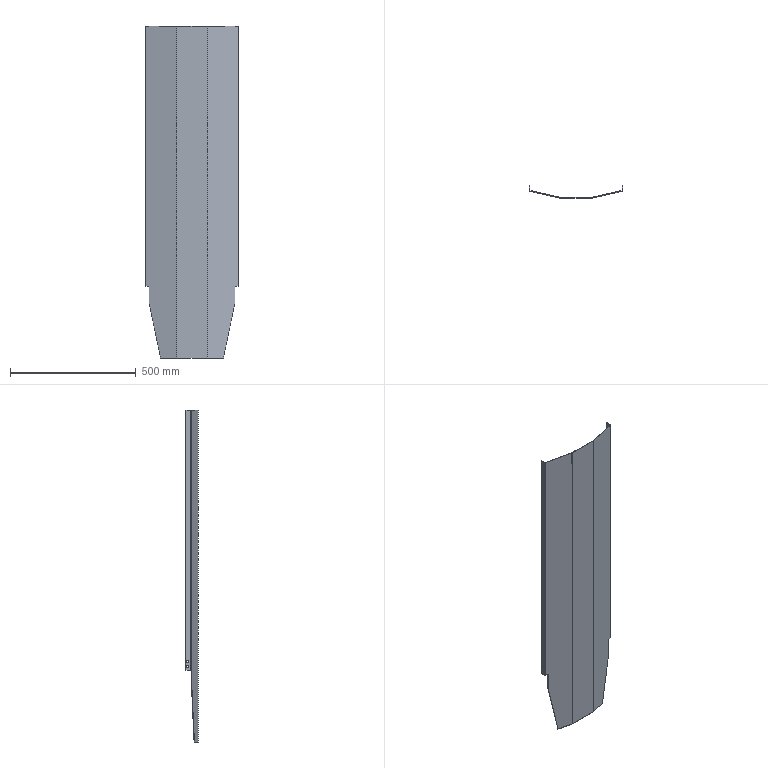Part | SolidWorks | features Fillet 3, ICE 2, FlatPattern 1, HoleWzd 1, SMBaseFlange 1, SheetMetal 1 | 1 solid | 48 faces | box 370 x 47.712 x 1320 mm | volume 619084 mm3 | plane 32 | cylinder 16 | commonest cylinder face diameters 6.6 x8 2 x4 4.4 x4
STEP:
#1=CARTESIAN_POINT('',(-183.8,55.014,-1016.7));
#2=VERTEX_POINT('',#1);
#3=CARTESIAN_POINT('',(-183.8,55.014,-1023.3));
#4=VERTEX_POINT('',#3);
#5=CARTESIAN_POINT('',(-183.8,55.014,-1020.));
#6=DIRECTION('',(1.,0.,0.));
#7=DIRECTION('',(0.,0.,-1.));
#8=AXIS2_PLACEMENT_3D('',#5,#6,#7);
#9=CIRCLE('',#8,3.3);
#10=EDGE_CURVE('',#2,#4,#9,.T.);
#11=ORIENTED_EDGE('',*,*,#10,.T.);
#12=CARTESIAN_POINT('',(-185.,55.014,-1023.3));
#13=VERTEX_POINT('',#12);
#14=CARTESIAN_POINT('',(-185.,55.014,-1023.3));
#15=DIRECTION('',(-1.,0.,0.));
#16=VECTOR('',#15,1000.);
#17=LINE('',#14,#16);
#18=EDGE_CURVE('',#4,#13,#17,.T.);
#19=ORIENTED_EDGE('',*,*,#18,.T.);
#20=CARTESIAN_POINT('',(-185.,55.014,-1016.7));
#21=VERTEX_POINT('',#20);
#22=CARTESIAN_POINT('',(-185.,55.014,-1020.));
#23=DIRECTION('',(-1.,0.,0.));
#24=DIRECTION('',(0.,0.,1.));
#25=AXIS2_PLACEMENT_3D('',#22,#23,#24);
#26=CIRCLE('',#25,3.3);
#27=EDGE_CURVE('',#13,#21,#26,.T.);
#28=ORIENTED_EDGE('',*,*,#27,.T.);
#29=CARTESIAN_POINT('',(-185.,55.014,-1016.7));
#30=DIRECTION('',(-1.,0.,0.));
#31=VECTOR('',#30,1000.);
#32=LINE('',#29,#31);
#33=EDGE_CURVE('',#2,#21,#32,.T.);
#34=ORIENTED_EDGE('',*,*,#33,.F.);
#35=EDGE_LOOP('',(#11,#19,#28,#34));
#36=FACE_OUTER_BOUND('',#35,.T.);
#37=CARTESIAN_POINT('',(-185.,55.014,-1020.));
#38=DIRECTION('',(-1.,0.,0.));
#39=DIRECTION('',(0.,0.,1.));
#40=AXIS2_PLACEMENT_3D('',#37,#38,#39);
#41=CYLINDRICAL_SURFACE('',#40,3.3);
#42=ADVANCED_FACE('',(#36),#41,.F.);
#43=CARTESIAN_POINT('',(185.,55.014,-1023.3));
#44=VERTEX_POINT('',#43);
#45=CARTESIAN_POINT('',(185.,55.014,-1016.7));
#46=VERTEX_POINT('',#45);
#47=CARTESIAN_POINT('',(185.,55.014,-1020.));
#48=DIRECTION('',(-1.,0.,0.));
#49=DIRECTION('',(0.,0.,1.));
#50=AXIS2_PLACEMENT_3D('',#47,#48,#49);
#51=CIRCLE('',#50,3.3);
#52=EDGE_CURVE('',#44,#46,#51,.T.);
#53=ORIENTED_EDGE('',*,*,#52,.F.);
#54=CARTESIAN_POINT('',(183.8,55.014,-1023.3));
#55=VERTEX_POINT('',#54);
#56=CARTESIAN_POINT('',(-185.,55.014,-1023.3));
#57=DIRECTION('',(-1.,0.,0.));
#58=VECTOR('',#57,1000.);
#59=LINE('',#56,#58);
#60=EDGE_CURVE('',#44,#55,#59,.T.);
#61=ORIENTED_EDGE('',*,*,#60,.T.);
#62=CARTESIAN_POINT('',(183.8,55.014,-1016.7));
#63=VERTEX_POINT('',#62);
#64=CARTESIAN_POINT('',(183.8,55.014,-1020.));
#65=DIRECTION('',(-1.,0.,0.));
#66=DIRECTION('',(0.,0.,1.));
#67=AXIS2_PLACEMENT_3D('',#64,#65,#66);
#68=CIRCLE('',#67,3.3);
#69=EDGE_CURVE('',#55,#63,#68,.T.);
#70=ORIENTED_EDGE('',*,*,#69,.T.);
#71=CARTESIAN_POINT('',(-185.,55.014,-1016.7));
#72=DIRECTION('',(-1.,0.,0.));
#73=VECTOR('',#72,1000.);
#74=LINE('',#71,#73);
#75=EDGE_CURVE('',#46,#63,#74,.T.);
#76=ORIENTED_EDGE('',*,*,#75,.F.);
#77=EDGE_LOOP('',(#53,#61,#70,#76));
#78=FACE_OUTER_BOUND('',#77,.T.);
#79=CARTESIAN_POINT('',(-185.,55.014,-1020.));
#80=DIRECTION('',(-1.,0.,0.));
#81=DIRECTION('',(0.,0.,1.));
#82=AXIS2_PLACEMENT_3D('',#79,#80,#81);
#83=CYLINDRICAL_SURFACE('',#82,3.3);
#84=ADVANCED_FACE('',(#78),#83,.F.);
#85=CARTESIAN_POINT('',(-183.8,55.014,-996.7));
#86=VERTEX_POINT('',#85);
#87=CARTESIAN_POINT('',(-183.8,55.014,-1003.3));
#88=VERTEX_POINT('',#87);
#89=CARTESIAN_POINT('',(-183.8,55.014,-1000.));
#90=DIRECTION('',(1.,0.,0.));
#91=DIRECTION('',(0.,0.,-1.));
#92=AXIS2_PLACEMENT_3D('',#89,#90,#91);
#93=CIRCLE('',#92,3.3);
#94=EDGE_CURVE('',#86,#88,#93,.T.);
#95=ORIENTED_EDGE('',*,*,#94,.T.);
#96=CARTESIAN_POINT('',(-185.,55.014,-1003.3));
#97=VERTEX_POINT('',#96);
#98=CARTESIAN_POINT('',(-185.,55.014,-1003.3));
#99=DIRECTION('',(-1.,0.,0.));
#100=VECTOR('',#99,1000.);
#101=LINE('',#98,#100);
#102=EDGE_CURVE('',#88,#97,#101,.T.);
#103=ORIENTED_EDGE('',*,*,#102,.T.);
#104=CARTESIAN_POINT('',(-185.,55.014,-996.7));
#105=VERTEX_POINT('',#104);
#106=CARTESIAN_POINT('',(-185.,55.014,-1000.));
#107=DIRECTION('',(-1.,0.,0.));
#108=DIRECTION('',(0.,0.,1.));
#109=AXIS2_PLACEMENT_3D('',#106,#107,#108);
#110=CIRCLE('',#109,3.3);
#111=EDGE_CURVE('',#97,#105,#110,.T.);
#112=ORIENTED_EDGE('',*,*,#111,.T.);
#113=CARTESIAN_POINT('',(-185.,55.014,-996.7));
#114=DIRECTION('',(-1.,0.,0.));
#115=VECTOR('',#114,1000.);
#116=LINE('',#113,#115);
#117=EDGE_CURVE('',#86,#105,#116,.T.);
#118=ORIENTED_EDGE('',*,*,#117,.F.);
#119=EDGE_LOOP('',(#95,#103,#112,#118));
#120=FACE_OUTER_BOUND('',#119,.T.);
#121=CARTESIAN_POINT('',(-185.,55.014,-1000.));
#122=DIRECTION('',(-1.,0.,0.));
#123=DIRECTION('',(0.,0.,1.));
#124=AXIS2_PLACEMENT_3D('',#121,#122,#123);
#125=CYLINDRICAL_SURFACE('',#124,3.3);
#126=ADVANCED_FACE('',(#120),#125,.F.);
#127=CARTESIAN_POINT('',(185.,55.014,-1003.3));
#128=VERTEX_POINT('',#127);
#129=CARTESIAN_POINT('',(185.,55.014,-996.7));
#130=VERTEX_POINT('',#129);
#131=CARTESIAN_POINT('',(185.,55.014,-1000.));
#132=DIRECTION('',(-1.,0.,0.));
#133=DIRECTION('',(0.,0.,1.));
#134=AXIS2_PLACEMENT_3D('',#131,#132,#133);
#135=CIRCLE('',#134,3.3);
#136=EDGE_CURVE('',#128,#130,#135,.T.);
#137=ORIENTED_EDGE('',*,*,#136,.F.);
#138=CARTESIAN_POINT('',(183.8,55.014,-1003.3));
#139=VERTEX_POINT('',#138);
#140=CARTESIAN_POINT('',(-185.,55.014,-1003.3));
#141=DIRECTION('',(-1.,0.,0.));
#142=VECTOR('',#141,1000.);
#143=LINE('',#140,#142);
#144=EDGE_CURVE('',#128,#139,#143,.T.);
#145=ORIENTED_EDGE('',*,*,#144,.T.);
#146=CARTESIAN_POINT('',(183.8,55.014,-996.7));
#147=VERTEX_POINT('',#146);
#148=CARTESIAN_POINT('',(183.8,55.014,-1000.));
#149=DIRECTION('',(-1.,0.,0.));
#150=DIRECTION('',(0.,0.,1.));
#151=AXIS2_PLACEMENT_3D('',#148,#149,#150);
#152=CIRCLE('',#151,3.3);
#153=EDGE_CURVE('',#139,#147,#152,.T.);
#154=ORIENTED_EDGE('',*,*,#153,.T.);
#155=CARTESIAN_POINT('',(-185.,55.014,-996.7));
#156=DIRECTION('',(-1.,0.,0.));
#157=VECTOR('',#156,1000.);
#158=LINE('',#155,#157);
#159=EDGE_CURVE('',#130,#147,#158,.T.);
#160=ORIENTED_EDGE('',*,*,#159,.F.);
#161=EDGE_LOOP('',(#137,#145,#154,#160));
#162=FACE_OUTER_BOUND('',#161,.T.);
#163=CARTESIAN_POINT('',(-185.,55.014,-1000.));
#164=DIRECTION('',(-1.,0.,0.));
#165=DIRECTION('',(0.,0.,1.));
#166=AXIS2_PLACEMENT_3D('',#163,#164,#165);
#167=CYLINDRICAL_SURFACE('',#166,3.3);
#168=ADVANCED_FACE('',(#162),#167,.F.);
#169=CARTESIAN_POINT('',(-60.235,13.354,-1320.));
#170=VERTEX_POINT('',#169);
#171=CARTESIAN_POINT('',(-125.,27.712,-1320.));
#172=VERTEX_POINT('',#171);
#173=CARTESIAN_POINT('',(-185.,41.014,-1320.));
#174=DIRECTION('',(-0.9763,0.2164,0.));
#175=VECTOR('',#174,1000.);
#176=LINE('',#173,#175);
#177=EDGE_CURVE('',#170,#172,#176,.T.);
#178=ORIENTED_EDGE('',*,*,#177,.T.);
#179=CARTESIAN_POINT('',(-125.,28.941,-1320.));
#180=VERTEX_POINT('',#179);
#181=CARTESIAN_POINT('',(-125.,13.302,-1320.));
#182=DIRECTION('',(0.,-1.,0.));
#183=VECTOR('',#182,1000.);
#184=LINE('',#181,#183);
#185=EDGE_CURVE('',#180,#172,#184,.T.);
#186=ORIENTED_EDGE('',*,*,#185,.F.);
#187=CARTESIAN_POINT('',(-59.976,14.525,-1320.));
#188=VERTEX_POINT('',#187);
#189=CARTESIAN_POINT('',(-184.74,42.185,-1320.));
#190=DIRECTION('',(-0.9763,0.2164,0.));
#191=VECTOR('',#190,1000.);
#192=LINE('',#189,#191);
#193=EDGE_CURVE('',#188,#180,#192,.T.);
#194=ORIENTED_EDGE('',*,*,#193,.F.);
#195=CARTESIAN_POINT('',(-59.976,14.525,-1320.));
#196=DIRECTION('',(-0.2164,-0.9763,0.));
#197=VECTOR('',#196,1000.);
#198=LINE('',#195,#197);
#199=EDGE_CURVE('',#188,#170,#198,.T.);
#200=ORIENTED_EDGE('',*,*,#199,.T.);
#201=EDGE_LOOP('',(#178,#186,#194,#200));
#202=FACE_OUTER_BOUND('',#201,.T.);
#203=CARTESIAN_POINT('',(-183.8,42.779,-1320.));
#204=DIRECTION('',(0.,0.,-1.));
#205=DIRECTION('',(-1.,0.,0.));
#206=AXIS2_PLACEMENT_3D('',#203,#204,#205);
#207=PLANE('',#206);
#208=ADVANCED_FACE('',(#202),#207,.T.);
#209=CARTESIAN_POINT('',(125.,28.941,-1320.));
#210=VERTEX_POINT('',#209);
#211=CARTESIAN_POINT('',(59.976,14.525,-1320.));
#212=VERTEX_POINT('',#211);
#213=CARTESIAN_POINT('',(59.74,14.473,-1320.));
#214=DIRECTION('',(-0.9763,-0.2164,0.));
#215=VECTOR('',#214,1000.);
#216=LINE('',#213,#215);
#217=EDGE_CURVE('',#210,#212,#216,.T.);
#218=ORIENTED_EDGE('',*,*,#217,.F.);
#219=CARTESIAN_POINT('',(125.,27.712,-1320.));
#220=VERTEX_POINT('',#219);
#221=CARTESIAN_POINT('',(125.,13.302,-1320.));
#222=DIRECTION('',(0.,-1.,0.));
#223=VECTOR('',#222,1000.);
#224=LINE('',#221,#223);
#225=EDGE_CURVE('',#210,#220,#224,.T.);
#226=ORIENTED_EDGE('',*,*,#225,.T.);
#227=CARTESIAN_POINT('',(60.235,13.354,-1320.));
#228=VERTEX_POINT('',#227);
#229=CARTESIAN_POINT('',(60.,13.302,-1320.));
#230=DIRECTION('',(-0.9763,-0.2164,0.));
#231=VECTOR('',#230,1000.);
#232=LINE('',#229,#231);
#233=EDGE_CURVE('',#220,#228,#232,.T.);
#234=ORIENTED_EDGE('',*,*,#233,.T.);
#235=CARTESIAN_POINT('',(60.235,13.354,-1320.));
#236=DIRECTION('',(-0.2164,0.9763,0.));
#237=VECTOR('',#236,1000.);
#238=LINE('',#235,#237);
#239=EDGE_CURVE('',#228,#212,#238,.T.);
#240=ORIENTED_EDGE('',*,*,#239,.T.);
#241=EDGE_LOOP('',(#218,#226,#234,#240));
#242=FACE_OUTER_BOUND('',#241,.T.);
#243=CARTESIAN_POINT('',(59.759,14.502,-1320.));
#244=DIRECTION('',(0.,0.,-1.));
#245=DIRECTION('',(-1.,0.,0.));
#246=AXIS2_PLACEMENT_3D('',#243,#244,#245);
#247=PLANE('',#246);
#248=ADVANCED_FACE('',(#242),#247,.T.);
#249=CARTESIAN_POINT('',(-185.,55.014,-1020.));
#250=DIRECTION('',(-1.,0.,0.));
#251=DIRECTION('',(0.,0.,1.));
#252=AXIS2_PLACEMENT_3D('',#249,#250,#251);
#253=CIRCLE('',#252,3.3);
#254=EDGE_CURVE('',#21,#13,#253,.T.);
#255=ORIENTED_EDGE('',*,*,#254,.F.);
#256=ORIENTED_EDGE('',*,*,#27,.F.);
#257=EDGE_LOOP('',(#255,#256));
#258=FACE_BOUND('',#257,.T.);
#259=CARTESIAN_POINT('',(-185.,55.014,-1000.));
#260=DIRECTION('',(-1.,0.,0.));
#261=DIRECTION('',(0.,0.,1.));
#262=AXIS2_PLACEMENT_3D('',#259,#260,#261);
#263=CIRCLE('',#262,3.3);
#264=EDGE_CURVE('',#105,#97,#263,.T.);
#265=ORIENTED_EDGE('',*,*,#264,.F.);
#266=ORIENTED_EDGE('',*,*,#111,.F.);
#267=EDGE_LOOP('',(#265,#266));
#268=FACE_BOUND('',#267,.T.);
#269=CARTESIAN_POINT('',(-185.,61.014,-1035.));
#270=VERTEX_POINT('',#269);
#271=CARTESIAN_POINT('',(-185.,42.779,-1035.));
#272=VERTEX_POINT('',#271);
#273=CARTESIAN_POINT('',(-185.,13.302,-1035.));
#274=DIRECTION('',(0.,-1.,0.));
#275=VECTOR('',#274,1000.);
#276=LINE('',#273,#275);
#277=EDGE_CURVE('',#270,#272,#276,.T.);
#278=ORIENTED_EDGE('',*,*,#277,.T.);
#279=CARTESIAN_POINT('',(-185.,42.779,0.));
#280=VERTEX_POINT('',#279);
#281=CARTESIAN_POINT('',(-185.,42.779,-1320.));
#282=DIRECTION('',(0.,0.,1.));
#283=VECTOR('',#282,1000.);
#284=LINE('',#281,#283);
#285=EDGE_CURVE('',#272,#280,#284,.T.);
#286=ORIENTED_EDGE('',*,*,#285,.T.);
#287=CARTESIAN_POINT('',(-185.,61.014,0.));
#288=VERTEX_POINT('',#287);
#289=CARTESIAN_POINT('',(-185.,41.014,0.));
#290=DIRECTION('',(0.,1.,0.));
#291=VECTOR('',#290,1000.);
#292=LINE('',#289,#291);
#293=EDGE_CURVE('',#280,#288,#292,.T.);
#294=ORIENTED_EDGE('',*,*,#293,.T.);
#295=CARTESIAN_POINT('',(-185.,61.014,-1320.));
#296=DIRECTION('',(0.,0.,1.));
#297=VECTOR('',#296,1000.);
#298=LINE('',#295,#297);
#299=EDGE_CURVE('',#270,#288,#298,.T.);
#300=ORIENTED_EDGE('',*,*,#299,.F.);
#301=EDGE_LOOP('',(#278,#286,#294,#300));
#302=FACE_OUTER_BOUND('',#301,.T.);
#303=CARTESIAN_POINT('',(-185.,41.014,-1320.));
#304=DIRECTION('',(1.,0.,0.));
#305=DIRECTION('',(0.,0.,-1.));
#306=AXIS2_PLACEMENT_3D('',#303,#304,#305);
#307=PLANE('',#306);
#308=ADVANCED_FACE('',(#258,#268,#302),#307,.F.);
#309=CARTESIAN_POINT('',(-183.8,61.014,-1035.));
#310=VERTEX_POINT('',#309);
#311=CARTESIAN_POINT('',(-183.8,61.014,0.));
#312=VERTEX_POINT('',#311);
#313=CARTESIAN_POINT('',(-183.8,61.014,-1320.));
#314=DIRECTION('',(0.,0.,1.));
#315=VECTOR('',#314,1000.);
#316=LINE('',#313,#315);
#317=EDGE_CURVE('',#310,#312,#316,.T.);
#318=ORIENTED_EDGE('',*,*,#317,.F.);
#319=CARTESIAN_POINT('',(-185.,61.014,-1035.));
#320=DIRECTION('',(1.,0.,0.));
#321=VECTOR('',#320,1000.);
#322=LINE('',#319,#321);
#323=EDGE_CURVE('',#270,#310,#322,.T.);
#324=ORIENTED_EDGE('',*,*,#323,.F.);
#325=ORIENTED_EDGE('',*,*,#299,.T.);
#326=CARTESIAN_POINT('',(-183.8,61.014,0.));
#327=DIRECTION('',(-1.,0.,0.));
#328=VECTOR('',#327,1000.);
#329=LINE('',#326,#328);
#330=EDGE_CURVE('',#312,#288,#329,.T.);
#331=ORIENTED_EDGE('',*,*,#330,.F.);
#332=EDGE_LOOP('',(#318,#324,#325,#331));
#333=FACE_OUTER_BOUND('',#332,.T.);
#334=CARTESIAN_POINT('',(-183.8,61.014,-1320.));
#335=DIRECTION('',(0.,1.,0.));
#336=DIRECTION('',(0.,0.,1.));
#337=AXIS2_PLACEMENT_3D('',#334,#335,#336);
#338=PLANE('',#337);
#339=ADVANCED_FACE('',(#333),#338,.T.);
#340=ORIENTED_EDGE('',*,*,#10,.F.);
#341=CARTESIAN_POINT('',(-183.8,55.014,-1020.));
#342=DIRECTION('',(1.,0.,0.));
#343=DIRECTION('',(0.,0.,-1.));
#344=AXIS2_PLACEMENT_3D('',#341,#342,#343);
#345=CIRCLE('',#344,3.3);
#346=EDGE_CURVE('',#4,#2,#345,.T.);
#347=ORIENTED_EDGE('',*,*,#346,.F.);
#348=EDGE_LOOP('',(#340,#347));
#349=FACE_BOUND('',#348,.T.);
#350=ORIENTED_EDGE('',*,*,#94,.F.);
#351=CARTESIAN_POINT('',(-183.8,55.014,-1000.));
#352=DIRECTION('',(1.,0.,0.));
#353=DIRECTION('',(0.,0.,-1.));
#354=AXIS2_PLACEMENT_3D('',#351,#352,#353);
#355=CIRCLE('',#354,3.3);
#356=EDGE_CURVE('',#88,#86,#355,.T.);
#357=ORIENTED_EDGE('',*,*,#356,.F.);
#358=EDGE_LOOP('',(#350,#357));
#359=FACE_BOUND('',#358,.T.);
#360=CARTESIAN_POINT('',(-183.8,42.779,-1035.));
#361=VERTEX_POINT('',#360);
#362=CARTESIAN_POINT('',(-183.8,42.779,0.));
#363=VERTEX_POINT('',#362);
#364=CARTESIAN_POINT('',(-183.8,42.779,-1320.));
#365=DIRECTION('',(0.,0.,1.));
#366=VECTOR('',#365,1000.);
#367=LINE('',#364,#366);
#368=EDGE_CURVE('',#361,#363,#367,.T.);
#369=ORIENTED_EDGE('',*,*,#368,.F.);
#370=CARTESIAN_POINT('',(-183.8,41.014,-1035.));
#371=DIRECTION('',(0.,1.,0.));
#372=VECTOR('',#371,1000.);
#373=LINE('',#370,#372);
#374=EDGE_CURVE('',#361,#310,#373,.T.);
#375=ORIENTED_EDGE('',*,*,#374,.T.);
#376=ORIENTED_EDGE('',*,*,#317,.T.);
#377=CARTESIAN_POINT('',(-183.8,41.014,0.));
#378=DIRECTION('',(0.,1.,0.));
#379=VECTOR('',#378,1000.);
#380=LINE('',#377,#379);
#381=EDGE_CURVE('',#363,#312,#380,.T.);
#382=ORIENTED_EDGE('',*,*,#381,.F.);
#383=EDGE_LOOP('',(#369,#375,#376,#382));
#384=FACE_OUTER_BOUND('',#383,.T.);
#385=CARTESIAN_POINT('',(-183.8,41.014,-1320.));
#386=DIRECTION('',(1.,0.,0.));
#387=DIRECTION('',(0.,0.,-1.));
#388=AXIS2_PLACEMENT_3D('',#385,#386,#387);
#389=PLANE('',#388);
#390=ADVANCED_FACE('',(#349,#359,#384),#389,.T.);
#391=CARTESIAN_POINT('',(-183.016,41.803,-1035.));
#392=VERTEX_POINT('',#391);
#393=CARTESIAN_POINT('',(-183.016,41.803,0.));
#394=VERTEX_POINT('',#393);
#395=CARTESIAN_POINT('',(-183.016,41.803,-1320.));
#396=DIRECTION('',(0.,0.,1.));
#397=VECTOR('',#396,1000.);
#398=LINE('',#395,#397);
#399=EDGE_CURVE('',#392,#394,#398,.T.);
#400=ORIENTED_EDGE('',*,*,#399,.F.);
#401=CARTESIAN_POINT('',(-182.8,42.779,-1035.));
#402=DIRECTION('',(0.,0.,-1.));
#403=DIRECTION('',(-1.,0.,0.));
#404=AXIS2_PLACEMENT_3D('',#401,#402,#403);
#405=CIRCLE('',#404,1.);
#406=EDGE_CURVE('',#392,#361,#405,.T.);
#407=ORIENTED_EDGE('',*,*,#406,.T.);
#408=ORIENTED_EDGE('',*,*,#368,.T.);
#409=CARTESIAN_POINT('',(-182.8,42.779,0.));
#410=DIRECTION('',(0.,0.,-1.));
#411=DIRECTION('',(1.,0.,0.));
#412=AXIS2_PLACEMENT_3D('',#409,#410,#411);
#413=CIRCLE('',#412,1.);
#414=EDGE_CURVE('',#394,#363,#413,.T.);
#415=ORIENTED_EDGE('',*,*,#414,.F.);
#416=EDGE_LOOP('',(#400,#407,#408,#415));
#417=FACE_OUTER_BOUND('',#416,.T.);
#418=CARTESIAN_POINT('',(-182.8,42.779,-1320.));
#419=DIRECTION('',(0.,0.,1.));
#420=DIRECTION('',(1.,0.,0.));
#421=AXIS2_PLACEMENT_3D('',#418,#419,#420);
#422=CYLINDRICAL_SURFACE('',#421,1.);
#423=ADVANCED_FACE('',(#417),#422,.F.);
#424=ORIENTED_EDGE('',*,*,#193,.T.);
#425=CARTESIAN_POINT('',(-170.,38.917,-1105.));
#426=VERTEX_POINT('',#425);
#427=CARTESIAN_POINT('',(-127.625,29.523,-1307.458));
#428=DIRECTION('',(-0.2047,0.04537,0.9778));
#429=VECTOR('',#428,1000.);
#430=LINE('',#427,#429);
#431=EDGE_CURVE('',#180,#426,#430,.T.);
#432=ORIENTED_EDGE('',*,*,#431,.T.);
#433=CARTESIAN_POINT('',(-170.,38.917,-1035.));
#434=VERTEX_POINT('',#433);
#435=CARTESIAN_POINT('',(-170.,38.917,-1320.));
#436=DIRECTION('',(0.,0.,1.));
#437=VECTOR('',#436,1000.);
#438=LINE('',#435,#437);
#439=EDGE_CURVE('',#426,#434,#438,.T.);
#440=ORIENTED_EDGE('',*,*,#439,.T.);
#441=CARTESIAN_POINT('',(-184.74,42.185,-1035.));
#442=DIRECTION('',(-0.9763,0.2164,0.));
#443=VECTOR('',#442,1000.);
#444=LINE('',#441,#443);
#445=EDGE_CURVE('',#434,#392,#444,.T.);
#446=ORIENTED_EDGE('',*,*,#445,.T.);
#447=ORIENTED_EDGE('',*,*,#399,.T.);
#448=CARTESIAN_POINT('',(-59.976,14.525,0.));
#449=VERTEX_POINT('',#448);
#450=CARTESIAN_POINT('',(-184.74,42.185,0.));
#451=DIRECTION('',(-0.9763,0.2164,0.));
#452=VECTOR('',#451,1000.);
#453=LINE('',#450,#452);
#454=EDGE_CURVE('',#449,#394,#453,.T.);
#455=ORIENTED_EDGE('',*,*,#454,.F.);
#456=CARTESIAN_POINT('',(-59.976,14.525,-1320.));
#457=DIRECTION('',(0.,0.,1.));
#458=VECTOR('',#457,1000.);
#459=LINE('',#456,#458);
#460=EDGE_CURVE('',#188,#449,#459,.T.);
#461=ORIENTED_EDGE('',*,*,#460,.F.);
#462=EDGE_LOOP('',(#424,#432,#440,#446,#447,#455,#461));
#463=FACE_OUTER_BOUND('',#462,.T.);
#464=CARTESIAN_POINT('',(-184.74,42.185,-1320.));
#465=DIRECTION('',(0.2164,0.9763,0.));
#466=DIRECTION('',(-0.9763,0.2164,0.));
#467=AXIS2_PLACEMENT_3D('',#464,#465,#466);
#468=PLANE('',#467);
#469=ADVANCED_FACE('',(#463),#468,.T.);
#470=CARTESIAN_POINT('',(183.016,41.803,-1035.));
#471=VERTEX_POINT('',#470);
#472=CARTESIAN_POINT('',(183.016,41.803,0.));
#473=VERTEX_POINT('',#472);
#474=CARTESIAN_POINT('',(183.016,41.803,-1320.));
#475=DIRECTION('',(0.,0.,1.));
#476=VECTOR('',#475,1000.);
#477=LINE('',#474,#476);
#478=EDGE_CURVE('',#471,#473,#477,.T.);
#479=ORIENTED_EDGE('',*,*,#478,.F.);
#480=CARTESIAN_POINT('',(170.,38.917,-1035.));
#481=VERTEX_POINT('',#480);
#482=CARTESIAN_POINT('',(59.74,14.473,-1035.));
#483=DIRECTION('',(-0.9763,-0.2164,0.));
#484=VECTOR('',#483,1000.);
#485=LINE('',#482,#484);
#486=EDGE_CURVE('',#471,#481,#485,.T.);
#487=ORIENTED_EDGE('',*,*,#486,.T.);
#488=CARTESIAN_POINT('',(170.,38.917,-1105.));
#489=VERTEX_POINT('',#488);
#490=CARTESIAN_POINT('',(170.,38.917,-1320.));
#491=DIRECTION('',(0.,0.,-1.));
#492=VECTOR('',#491,1000.);
#493=LINE('',#490,#492);
#494=EDGE_CURVE('',#481,#489,#493,.T.);
#495=ORIENTED_EDGE('',*,*,#494,.T.);
#496=CARTESIAN_POINT('',(122.132,28.305,-1333.701));
#497=DIRECTION('',(-0.2047,-0.04537,-0.9778));
#498=VECTOR('',#497,1000.);
#499=LINE('',#496,#498);
#500=EDGE_CURVE('',#489,#210,#499,.T.);
#501=ORIENTED_EDGE('',*,*,#500,.T.);
#502=ORIENTED_EDGE('',*,*,#217,.T.);
#503=CARTESIAN_POINT('',(59.976,14.525,0.));
#504=VERTEX_POINT('',#503);
#505=CARTESIAN_POINT('',(59.976,14.525,-1320.));
#506=DIRECTION('',(0.,0.,1.));
#507=VECTOR('',#506,1000.);
#508=LINE('',#505,#507);
#509=EDGE_CURVE('',#212,#504,#508,.T.);
#510=ORIENTED_EDGE('',*,*,#509,.T.);
#511=CARTESIAN_POINT('',(59.74,14.473,0.));
#512=DIRECTION('',(-0.9763,-0.2164,0.));
#513=VECTOR('',#512,1000.);
#514=LINE('',#511,#513);
#515=EDGE_CURVE('',#473,#504,#514,.T.);
#516=ORIENTED_EDGE('',*,*,#515,.F.);
#517=EDGE_LOOP('',(#479,#487,#495,#501,#502,#510,#516));
#518=FACE_OUTER_BOUND('',#517,.T.);
#519=CARTESIAN_POINT('',(59.74,14.473,-1320.));
#520=DIRECTION('',(-0.2164,0.9763,0.));
#521=DIRECTION('',(-0.9763,-0.2164,0.));
#522=AXIS2_PLACEMENT_3D('',#519,#520,#521);
#523=PLANE('',#522);
#524=ADVANCED_FACE('',(#518),#523,.T.);
#525=CARTESIAN_POINT('',(183.8,42.779,-1035.));
#526=VERTEX_POINT('',#525);
#527=CARTESIAN_POINT('',(183.8,42.779,0.));
#528=VERTEX_POINT('',#527);
#529=CARTESIAN_POINT('',(183.8,42.779,-1320.));
#530=DIRECTION('',(0.,0.,1.));
#531=VECTOR('',#530,1000.);
#532=LINE('',#529,#531);
#533=EDGE_CURVE('',#526,#528,#532,.T.);
#534=ORIENTED_EDGE('',*,*,#533,.F.);
#535=CARTESIAN_POINT('',(182.8,42.779,-1035.));
#536=DIRECTION('',(0.,0.,-1.));
#537=DIRECTION('',(-1.,0.,0.));
#538=AXIS2_PLACEMENT_3D('',#535,#536,#537);
#539=CIRCLE('',#538,1.);
#540=EDGE_CURVE('',#526,#471,#539,.T.);
#541=ORIENTED_EDGE('',*,*,#540,.T.);
#542=ORIENTED_EDGE('',*,*,#478,.T.);
#543=CARTESIAN_POINT('',(182.8,42.779,0.));
#544=DIRECTION('',(0.,0.,-1.));
#545=DIRECTION('',(1.,0.,0.));
#546=AXIS2_PLACEMENT_3D('',#543,#544,#545);
#547=CIRCLE('',#546,1.);
#548=EDGE_CURVE('',#528,#473,#547,.T.);
#549=ORIENTED_EDGE('',*,*,#548,.F.);
#550=EDGE_LOOP('',(#534,#541,#542,#549));
#551=FACE_OUTER_BOUND('',#550,.T.);
#552=CARTESIAN_POINT('',(182.8,42.779,-1320.));
#553=DIRECTION('',(0.,0.,1.));
#554=DIRECTION('',(1.,0.,0.));
#555=AXIS2_PLACEMENT_3D('',#552,#553,#554);
#556=CYLINDRICAL_SURFACE('',#555,1.);
#557=ADVANCED_FACE('',(#551),#556,.F.);
#558=CARTESIAN_POINT('',(183.8,55.014,-1020.));
#559=DIRECTION('',(-1.,0.,0.));
#560=DIRECTION('',(0.,0.,1.));
#561=AXIS2_PLACEMENT_3D('',#558,#559,#560);
#562=CIRCLE('',#561,3.3);
#563=EDGE_CURVE('',#63,#55,#562,.T.);
#564=ORIENTED_EDGE('',*,*,#563,.F.);
#565=ORIENTED_EDGE('',*,*,#69,.F.);
#566=EDGE_LOOP('',(#564,#565));
#567=FACE_BOUND('',#566,.T.);
#568=CARTESIAN_POINT('',(183.8,55.014,-1000.));
#569=DIRECTION('',(-1.,0.,0.));
#570=DIRECTION('',(0.,0.,1.));
#571=AXIS2_PLACEMENT_3D('',#568,#569,#570);
#572=CIRCLE('',#571,3.3);
#573=EDGE_CURVE('',#147,#139,#572,.T.);
#574=ORIENTED_EDGE('',*,*,#573,.F.);
#575=ORIENTED_EDGE('',*,*,#153,.F.);
#576=EDGE_LOOP('',(#574,#575));
#577=FACE_BOUND('',#576,.T.);
#578=CARTESIAN_POINT('',(183.8,61.014,-1035.));
#579=VERTEX_POINT('',#578);
#580=CARTESIAN_POINT('',(183.8,61.014,0.));
#581=VERTEX_POINT('',#580);
#582=CARTESIAN_POINT('',(183.8,61.014,-1320.));
#583=DIRECTION('',(0.,0.,1.));
#584=VECTOR('',#583,1000.);
#585=LINE('',#582,#584);
#586=EDGE_CURVE('',#579,#581,#585,.T.);
#587=ORIENTED_EDGE('',*,*,#586,.F.);
#588=CARTESIAN_POINT('',(183.8,41.014,-1035.));
#589=DIRECTION('',(0.,-1.,0.));
#590=VECTOR('',#589,1000.);
#591=LINE('',#588,#590);
#592=EDGE_CURVE('',#579,#526,#591,.T.);
#593=ORIENTED_EDGE('',*,*,#592,.T.);
#594=ORIENTED_EDGE('',*,*,#533,.T.);
#595=CARTESIAN_POINT('',(183.8,41.014,0.));
#596=DIRECTION('',(0.,-1.,0.));
#597=VECTOR('',#596,1000.);
#598=LINE('',#595,#597);
#599=EDGE_CURVE('',#581,#528,#598,.T.);
#600=ORIENTED_EDGE('',*,*,#599,.F.);
#601=EDGE_LOOP('',(#587,#593,#594,#600));
#602=FACE_OUTER_BOUND('',#601,.T.);
#603=CARTESIAN_POINT('',(183.8,41.014,-1320.));
#604=DIRECTION('',(-1.,0.,0.));
#605=DIRECTION('',(0.,0.,1.));
#606=AXIS2_PLACEMENT_3D('',#603,#604,#605);
#607=PLANE('',#606);
#608=ADVANCED_FACE('',(#567,#577,#602),#607,.T.);
#609=CARTESIAN_POINT('',(185.,61.014,-1035.));
#610=VERTEX_POINT('',#609);
#611=CARTESIAN_POINT('',(185.,61.014,0.));
#612=VERTEX_POINT('',#611);
#613=CARTESIAN_POINT('',(185.,61.014,-1320.));
#614=DIRECTION('',(0.,0.,1.));
#615=VECTOR('',#614,1000.);
#616=LINE('',#613,#615);
#617=EDGE_CURVE('',#610,#612,#616,.T.);
#618=ORIENTED_EDGE('',*,*,#617,.F.);
#619=CARTESIAN_POINT('',(180.,61.014,-1035.));
#620=DIRECTION('',(1.,0.,0.));
#621=VECTOR('',#620,1000.);
#622=LINE('',#619,#621);
#623=EDGE_CURVE('',#579,#610,#622,.T.);
#624=ORIENTED_EDGE('',*,*,#623,.F.);
#625=ORIENTED_EDGE('',*,*,#586,.T.);
#626=CARTESIAN_POINT('',(185.,61.014,0.));
#627=DIRECTION('',(-1.,0.,0.));
#628=VECTOR('',#627,1000.);
#629=LINE('',#626,#628);
#630=EDGE_CURVE('',#612,#581,#629,.T.);
#631=ORIENTED_EDGE('',*,*,#630,.F.);
#632=EDGE_LOOP('',(#618,#624,#625,#631));
#633=FACE_OUTER_BOUND('',#632,.T.);
#634=CARTESIAN_POINT('',(185.,61.014,-1320.));
#635=DIRECTION('',(0.,1.,0.));
#636=DIRECTION('',(0.,0.,1.));
#637=AXIS2_PLACEMENT_3D('',#634,#635,#636);
#638=PLANE('',#637);
#639=ADVANCED_FACE('',(#633),#638,.T.);
#640=CARTESIAN_POINT('',(185.,55.014,-1020.));
#641=DIRECTION('',(-1.,0.,0.));
#642=DIRECTION('',(0.,0.,1.));
#643=AXIS2_PLACEMENT_3D('',#640,#641,#642);
#644=CIRCLE('',#643,3.3);
#645=EDGE_CURVE('',#46,#44,#644,.T.);
#646=ORIENTED_EDGE('',*,*,#645,.T.);
#647=ORIENTED_EDGE('',*,*,#52,.T.);
#648=EDGE_LOOP('',(#646,#647));
#649=FACE_BOUND('',#648,.T.);
#650=CARTESIAN_POINT('',(185.,55.014,-1000.));
#651=DIRECTION('',(-1.,0.,0.));
#652=DIRECTION('',(0.,0.,1.));
#653=AXIS2_PLACEMENT_3D('',#650,#651,#652);
#654=CIRCLE('',#653,3.3);
#655=EDGE_CURVE('',#130,#128,#654,.T.);
#656=ORIENTED_EDGE('',*,*,#655,.T.);
#657=ORIENTED_EDGE('',*,*,#136,.T.);
#658=EDGE_LOOP('',(#656,#657));
#659=FACE_BOUND('',#658,.T.);
#660=CARTESIAN_POINT('',(185.,42.779,-1035.));
#661=VERTEX_POINT('',#660);
#662=CARTESIAN_POINT('',(185.,13.302,-1035.));
#663=DIRECTION('',(0.,-1.,0.));
#664=VECTOR('',#663,1000.);
#665=LINE('',#662,#664);
#666=EDGE_CURVE('',#610,#661,#665,.T.);
#667=ORIENTED_EDGE('',*,*,#666,.F.);
#668=ORIENTED_EDGE('',*,*,#617,.T.);
#669=CARTESIAN_POINT('',(185.,42.779,0.));
#670=VERTEX_POINT('',#669);
#671=CARTESIAN_POINT('',(185.,41.014,0.));
#672=DIRECTION('',(0.,-1.,0.));
#673=VECTOR('',#672,1000.);
#674=LINE('',#671,#673);
#675=EDGE_CURVE('',#612,#670,#674,.T.);
#676=ORIENTED_EDGE('',*,*,#675,.T.);
#677=CARTESIAN_POINT('',(185.,42.779,-1320.));
#678=DIRECTION('',(0.,0.,1.));
#679=VECTOR('',#678,1000.);
#680=LINE('',#677,#679);
#681=EDGE_CURVE('',#661,#670,#680,.T.);
#682=ORIENTED_EDGE('',*,*,#681,.F.);
#683=EDGE_LOOP('',(#667,#668,#676,#682));
#684=FACE_OUTER_BOUND('',#683,.T.);
#685=CARTESIAN_POINT('',(185.,41.014,-1320.));
#686=DIRECTION('',(-1.,0.,0.));
#687=DIRECTION('',(0.,0.,1.));
#688=AXIS2_PLACEMENT_3D('',#685,#686,#687);
#689=PLANE('',#688);
#690=ADVANCED_FACE('',(#649,#659,#684),#689,.F.);
#691=CARTESIAN_POINT('',(183.276,40.631,-1035.));
#692=VERTEX_POINT('',#691);
#693=CARTESIAN_POINT('',(182.8,42.779,-1035.));
#694=DIRECTION('',(0.,0.,-1.));
#695=DIRECTION('',(-1.,0.,0.));
#696=AXIS2_PLACEMENT_3D('',#693,#694,#695);
#697=CIRCLE('',#696,2.2);
#698=EDGE_CURVE('',#661,#692,#697,.T.);
#699=ORIENTED_EDGE('',*,*,#698,.F.);
#700=ORIENTED_EDGE('',*,*,#681,.T.);
#701=CARTESIAN_POINT('',(183.276,40.631,0.));
#702=VERTEX_POINT('',#701);
#703=CARTESIAN_POINT('',(182.8,42.779,0.));
#704=DIRECTION('',(0.,0.,-1.));
#705=DIRECTION('',(-1.,0.,0.));
#706=AXIS2_PLACEMENT_3D('',#703,#704,#705);
#707=CIRCLE('',#706,2.2);
#708=EDGE_CURVE('',#670,#702,#707,.T.);
#709=ORIENTED_EDGE('',*,*,#708,.T.);
#710=CARTESIAN_POINT('',(183.276,40.631,-1320.));
#711=DIRECTION('',(0.,0.,1.));
#712=VECTOR('',#711,1000.);
#713=LINE('',#710,#712);
#714=EDGE_CURVE('',#692,#702,#713,.T.);
#715=ORIENTED_EDGE('',*,*,#714,.F.);
#716=EDGE_LOOP('',(#699,#700,#709,#715));
#717=FACE_OUTER_BOUND('',#716,.T.);
#718=CARTESIAN_POINT('',(182.8,42.779,-1320.));
#719=DIRECTION('',(0.,0.,1.));
#720=DIRECTION('',(1.,0.,0.));
#721=AXIS2_PLACEMENT_3D('',#718,#719,#720);
#722=CYLINDRICAL_SURFACE('',#721,2.2);
#723=ADVANCED_FACE('',(#717),#722,.T.);
#724=CARTESIAN_POINT('',(170.,37.688,-1035.));
#725=VERTEX_POINT('',#724);
#726=CARTESIAN_POINT('',(60.,13.302,-1035.));
#727=DIRECTION('',(-0.9763,-0.2164,0.));
#728=VECTOR('',#727,1000.);
#729=LINE('',#726,#728);
#730=EDGE_CURVE('',#692,#725,#729,.T.);
#731=ORIENTED_EDGE('',*,*,#730,.F.);
#732=ORIENTED_EDGE('',*,*,#714,.T.);
#733=CARTESIAN_POINT('',(60.235,13.354,0.));
#734=VERTEX_POINT('',#733);
#735=CARTESIAN_POINT('',(60.,13.302,0.));
#736=DIRECTION('',(-0.9763,-0.2164,0.));
#737=VECTOR('',#736,1000.);
#738=LINE('',#735,#737);
#739=EDGE_CURVE('',#702,#734,#738,.T.);
#740=ORIENTED_EDGE('',*,*,#739,.T.);
#741=CARTESIAN_POINT('',(60.235,13.354,-1320.));
#742=DIRECTION('',(0.,0.,1.));
#743=VECTOR('',#742,1000.);
#744=LINE('',#741,#743);
#745=EDGE_CURVE('',#228,#734,#744,.T.);
#746=ORIENTED_EDGE('',*,*,#745,.F.);
#747=ORIENTED_EDGE('',*,*,#233,.F.);
#748=CARTESIAN_POINT('',(170.,37.688,-1105.));
#749=VERTEX_POINT('',#748);
#750=CARTESIAN_POINT('',(122.144,27.079,-1333.646));
#751=DIRECTION('',(-0.2047,-0.04537,-0.9778));
#752=VECTOR('',#751,1000.);
#753=LINE('',#750,#752);
#754=EDGE_CURVE('',#749,#220,#753,.T.);
#755=ORIENTED_EDGE('',*,*,#754,.F.);
#756=CARTESIAN_POINT('',(170.,37.688,-1320.));
#757=DIRECTION('',(0.,0.,-1.));
#758=VECTOR('',#757,1000.);
#759=LINE('',#756,#758);
#760=EDGE_CURVE('',#725,#749,#759,.T.);
#761=ORIENTED_EDGE('',*,*,#760,.F.);
#762=EDGE_LOOP('',(#731,#732,#740,#746,#747,#755,#761));
#763=FACE_OUTER_BOUND('',#762,.T.);
#764=CARTESIAN_POINT('',(60.,13.302,-1320.));
#765=DIRECTION('',(-0.2164,0.9763,0.));
#766=DIRECTION('',(-0.9763,-0.2164,0.));
#767=AXIS2_PLACEMENT_3D('',#764,#765,#766);
#768=PLANE('',#767);
#769=ADVANCED_FACE('',(#763),#768,.F.);
#770=CARTESIAN_POINT('',(-170.,37.688,-1105.));
#771=VERTEX_POINT('',#770);
#772=CARTESIAN_POINT('',(-127.636,28.296,-1307.404));
#773=DIRECTION('',(-0.2047,0.04537,0.9778));
#774=VECTOR('',#773,1000.);
#775=LINE('',#772,#774);
#776=EDGE_CURVE('',#172,#771,#775,.T.);
#777=ORIENTED_EDGE('',*,*,#776,.F.);
#778=ORIENTED_EDGE('',*,*,#177,.F.);
#779=CARTESIAN_POINT('',(-60.235,13.354,0.));
#780=VERTEX_POINT('',#779);
#781=CARTESIAN_POINT('',(-60.235,13.354,-1320.));
#782=DIRECTION('',(0.,0.,1.));
#783=VECTOR('',#782,1000.);
#784=LINE('',#781,#783);
#785=EDGE_CURVE('',#170,#780,#784,.T.);
#786=ORIENTED_EDGE('',*,*,#785,.T.);
#787=CARTESIAN_POINT('',(-183.276,40.631,0.));
#788=VERTEX_POINT('',#787);
#789=CARTESIAN_POINT('',(-185.,41.014,0.));
#790=DIRECTION('',(-0.9763,0.2164,0.));
#791=VECTOR('',#790,1000.);
#792=LINE('',#789,#791);
#793=EDGE_CURVE('',#780,#788,#792,.T.);
#794=ORIENTED_EDGE('',*,*,#793,.T.);
#795=CARTESIAN_POINT('',(-183.276,40.631,-1035.));
#796=VERTEX_POINT('',#795);
#797=CARTESIAN_POINT('',(-183.276,40.631,-1320.));
#798=DIRECTION('',(0.,0.,1.));
#799=VECTOR('',#798,1000.);
#800=LINE('',#797,#799);
#801=EDGE_CURVE('',#796,#788,#800,.T.);
#802=ORIENTED_EDGE('',*,*,#801,.F.);
#803=CARTESIAN_POINT('',(-170.,37.688,-1035.));
#804=VERTEX_POINT('',#803);
#805=CARTESIAN_POINT('',(-185.,41.014,-1035.));
#806=DIRECTION('',(-0.9763,0.2164,0.));
#807=VECTOR('',#806,1000.);
#808=LINE('',#805,#807);
#809=EDGE_CURVE('',#804,#796,#808,.T.);
#810=ORIENTED_EDGE('',*,*,#809,.F.);
#811=CARTESIAN_POINT('',(-170.,37.688,-1320.));
#812=DIRECTION('',(0.,0.,1.));
#813=VECTOR('',#812,1000.);
#814=LINE('',#811,#813);
#815=EDGE_CURVE('',#771,#804,#814,.T.);
#816=ORIENTED_EDGE('',*,*,#815,.F.);
#817=EDGE_LOOP('',(#777,#778,#786,#794,#802,#810,#816));
#818=FACE_OUTER_BOUND('',#817,.T.);
#819=CARTESIAN_POINT('',(-185.,41.014,-1320.));
#820=DIRECTION('',(0.2164,0.9763,0.));
#821=DIRECTION('',(-0.9763,0.2164,0.));
#822=AXIS2_PLACEMENT_3D('',#819,#820,#821);
#823=PLANE('',#822);
#824=ADVANCED_FACE('',(#818),#823,.F.);
#825=CARTESIAN_POINT('',(-182.8,42.779,-1035.));
#826=DIRECTION('',(0.,0.,-1.));
#827=DIRECTION('',(-1.,0.,0.));
#828=AXIS2_PLACEMENT_3D('',#825,#826,#827);
#829=CIRCLE('',#828,2.2);
#830=EDGE_CURVE('',#796,#272,#829,.T.);
#831=ORIENTED_EDGE('',*,*,#830,.F.);
#832=ORIENTED_EDGE('',*,*,#801,.T.);
#833=CARTESIAN_POINT('',(-182.8,42.779,0.));
#834=DIRECTION('',(0.,0.,-1.));
#835=DIRECTION('',(-1.,0.,0.));
#836=AXIS2_PLACEMENT_3D('',#833,#834,#835);
#837=CIRCLE('',#836,2.2);
#838=EDGE_CURVE('',#788,#280,#837,.T.);
#839=ORIENTED_EDGE('',*,*,#838,.T.);
#840=ORIENTED_EDGE('',*,*,#285,.F.);
#841=EDGE_LOOP('',(#831,#832,#839,#840));
#842=FACE_OUTER_BOUND('',#841,.T.);
#843=CARTESIAN_POINT('',(-182.8,42.779,-1320.));
#844=DIRECTION('',(0.,0.,1.));
#845=DIRECTION('',(1.,0.,0.));
#846=AXIS2_PLACEMENT_3D('',#843,#844,#845);
#847=CYLINDRICAL_SURFACE('',#846,2.2);
#848=ADVANCED_FACE('',(#842),#847,.T.);
#849=CARTESIAN_POINT('',(-185.,42.779,0.));
#850=DIRECTION('',(1.,0.,0.));
#851=VECTOR('',#850,1000.);
#852=LINE('',#849,#851);
#853=EDGE_CURVE('',#280,#363,#852,.T.);
#854=ORIENTED_EDGE('',*,*,#853,.F.);
#855=ORIENTED_EDGE('',*,*,#838,.F.);
#856=CARTESIAN_POINT('',(-183.016,41.803,0.));
#857=DIRECTION('',(-0.2164,-0.9763,0.));
#858=VECTOR('',#857,1000.);
#859=LINE('',#856,#858);
#860=EDGE_CURVE('',#394,#788,#859,.T.);
#861=ORIENTED_EDGE('',*,*,#860,.F.);
#862=ORIENTED_EDGE('',*,*,#414,.T.);
#863=EDGE_LOOP('',(#854,#855,#861,#862));
#864=FACE_OUTER_BOUND('',#863,.T.);
#865=CARTESIAN_POINT('',(-185.,42.779,0.));
#866=DIRECTION('',(0.,0.,1.));
#867=DIRECTION('',(1.,0.,0.));
#868=AXIS2_PLACEMENT_3D('',#865,#866,#867);
#869=PLANE('',#868);
#870=ADVANCED_FACE('',(#864),#869,.T.);
#871=ORIENTED_EDGE('',*,*,#293,.F.);
#872=ORIENTED_EDGE('',*,*,#853,.T.);
#873=ORIENTED_EDGE('',*,*,#381,.T.);
#874=ORIENTED_EDGE('',*,*,#330,.T.);
#875=EDGE_LOOP('',(#871,#872,#873,#874));
#876=FACE_OUTER_BOUND('',#875,.T.);
#877=CARTESIAN_POINT('',(-183.016,41.803,0.));
#878=DIRECTION('',(0.,0.,1.));
#879=DIRECTION('',(1.,0.,0.));
#880=AXIS2_PLACEMENT_3D('',#877,#878,#879);
#881=PLANE('',#880);
#882=ADVANCED_FACE('',(#876),#881,.T.);
#883=CARTESIAN_POINT('',(-59.759,13.302,-1320.));
#884=VERTEX_POINT('',#883);
#885=CARTESIAN_POINT('',(-59.759,14.502,-1320.));
#886=VERTEX_POINT('',#885);
#887=CARTESIAN_POINT('',(-59.759,13.302,-1320.));
#888=DIRECTION('',(0.,1.,0.));
#889=VECTOR('',#888,1000.);
#890=LINE('',#887,#889);
#891=EDGE_CURVE('',#884,#886,#890,.T.);
#892=ORIENTED_EDGE('',*,*,#891,.F.);
#893=CARTESIAN_POINT('',(-59.759,15.502,-1320.));
#894=DIRECTION('',(0.,0.,-1.));
#895=DIRECTION('',(-1.,0.,0.));
#896=AXIS2_PLACEMENT_3D('',#893,#894,#895);
#897=CIRCLE('',#896,2.2);
#898=EDGE_CURVE('',#884,#170,#897,.T.);
#899=ORIENTED_EDGE('',*,*,#898,.T.);
#900=ORIENTED_EDGE('',*,*,#199,.F.);
#901=CARTESIAN_POINT('',(-59.759,15.502,-1320.));
#902=DIRECTION('',(0.,0.,-1.));
#903=DIRECTION('',(1.,0.,0.));
#904=AXIS2_PLACEMENT_3D('',#901,#902,#903);
#905=CIRCLE('',#904,1.);
#906=EDGE_CURVE('',#886,#188,#905,.T.);
#907=ORIENTED_EDGE('',*,*,#906,.F.);
#908=EDGE_LOOP('',(#892,#899,#900,#907));
#909=FACE_OUTER_BOUND('',#908,.T.);
#910=CARTESIAN_POINT('',(-59.759,13.302,-1320.));
#911=DIRECTION('',(0.,0.,-1.));
#912=DIRECTION('',(-1.,0.,0.));
#913=AXIS2_PLACEMENT_3D('',#910,#911,#912);
#914=PLANE('',#913);
#915=ADVANCED_FACE('',(#909),#914,.T.);
#916=CARTESIAN_POINT('',(59.759,13.302,-1320.));
#917=VERTEX_POINT('',#916);
#918=CARTESIAN_POINT('',(-60.,13.302,-1320.));
#919=DIRECTION('',(-1.,0.,0.));
#920=VECTOR('',#919,1000.);
#921=LINE('',#918,#920);
#922=EDGE_CURVE('',#917,#884,#921,.T.);
#923=ORIENTED_EDGE('',*,*,#922,.T.);
#924=ORIENTED_EDGE('',*,*,#891,.T.);
#925=CARTESIAN_POINT('',(59.759,14.502,-1320.));
#926=VERTEX_POINT('',#925);
#927=CARTESIAN_POINT('',(-60.,14.502,-1320.));
#928=DIRECTION('',(-1.,0.,0.));
#929=VECTOR('',#928,1000.);
#930=LINE('',#927,#929);
#931=EDGE_CURVE('',#926,#886,#930,.T.);
#932=ORIENTED_EDGE('',*,*,#931,.F.);
#933=CARTESIAN_POINT('',(59.759,14.502,-1320.));
#934=DIRECTION('',(0.,-1.,0.));
#935=VECTOR('',#934,1000.);
#936=LINE('',#933,#935);
#937=EDGE_CURVE('',#926,#917,#936,.T.);
#938=ORIENTED_EDGE('',*,*,#937,.T.);
#939=EDGE_LOOP('',(#923,#924,#932,#938));
#940=FACE_OUTER_BOUND('',#939,.T.);
#941=CARTESIAN_POINT('',(-59.976,14.525,-1320.));
#942=DIRECTION('',(0.,0.,-1.));
#943=DIRECTION('',(-1.,0.,0.));
#944=AXIS2_PLACEMENT_3D('',#941,#942,#943);
#945=PLANE('',#944);
#946=ADVANCED_FACE('',(#940),#945,.T.);
#947=CARTESIAN_POINT('',(-60.235,13.354,0.));
#948=DIRECTION('',(0.2164,0.9763,0.));
#949=VECTOR('',#948,1000.);
#950=LINE('',#947,#949);
#951=EDGE_CURVE('',#780,#449,#950,.T.);
#952=ORIENTED_EDGE('',*,*,#951,.F.);
#953=CARTESIAN_POINT('',(-59.759,13.302,0.));
#954=VERTEX_POINT('',#953);
#955=CARTESIAN_POINT('',(-59.759,15.502,0.));
#956=DIRECTION('',(0.,0.,-1.));
#957=DIRECTION('',(-1.,0.,0.));
#958=AXIS2_PLACEMENT_3D('',#955,#956,#957);
#959=CIRCLE('',#958,2.2);
#960=EDGE_CURVE('',#954,#780,#959,.T.);
#961=ORIENTED_EDGE('',*,*,#960,.F.);
#962=CARTESIAN_POINT('',(-59.759,14.502,0.));
#963=VERTEX_POINT('',#962);
#964=CARTESIAN_POINT('',(-59.759,14.502,0.));
#965=DIRECTION('',(0.,-1.,0.));
#966=VECTOR('',#965,1000.);
#967=LINE('',#964,#966);
#968=EDGE_CURVE('',#963,#954,#967,.T.);
#969=ORIENTED_EDGE('',*,*,#968,.F.);
#970=CARTESIAN_POINT('',(-59.759,15.502,0.));
#971=DIRECTION('',(0.,0.,-1.));
#972=DIRECTION('',(1.,0.,0.));
#973=AXIS2_PLACEMENT_3D('',#970,#971,#972);
#974=CIRCLE('',#973,1.);
#975=EDGE_CURVE('',#963,#449,#974,.T.);
#976=ORIENTED_EDGE('',*,*,#975,.T.);
#977=EDGE_LOOP('',(#952,#961,#969,#976));
#978=FACE_OUTER_BOUND('',#977,.T.);
#979=CARTESIAN_POINT('',(-60.235,13.354,0.));
#980=DIRECTION('',(0.,0.,1.));
#981=DIRECTION('',(1.,0.,0.));
#982=AXIS2_PLACEMENT_3D('',#979,#980,#981);
#983=PLANE('',#982);
#984=ADVANCED_FACE('',(#978),#983,.T.);
#985=ORIENTED_EDGE('',*,*,#793,.F.);
#986=ORIENTED_EDGE('',*,*,#951,.T.);
#987=ORIENTED_EDGE('',*,*,#454,.T.);
#988=ORIENTED_EDGE('',*,*,#860,.T.);
#989=EDGE_LOOP('',(#985,#986,#987,#988));
#990=FACE_OUTER_BOUND('',#989,.T.);
#991=CARTESIAN_POINT('',(-59.759,14.502,0.));
#992=DIRECTION('',(0.,0.,1.));
#993=DIRECTION('',(1.,0.,0.));
#994=AXIS2_PLACEMENT_3D('',#991,#992,#993);
#995=PLANE('',#994);
#996=ADVANCED_FACE('',(#990),#995,.T.);
#997=ORIENTED_EDGE('',*,*,#239,.F.);
#998=CARTESIAN_POINT('',(59.759,15.502,-1320.));
#999=DIRECTION('',(0.,0.,-1.));
#1000=DIRECTION('',(-1.,0.,0.));
#1001=AXIS2_PLACEMENT_3D('',#998,#999,#1000);
#1002=CIRCLE('',#1001,2.2);
#1003=EDGE_CURVE('',#228,#917,#1002,.T.);
#1004=ORIENTED_EDGE('',*,*,#1003,.T.);
#1005=ORIENTED_EDGE('',*,*,#937,.F.);
#1006=CARTESIAN_POINT('',(59.759,15.502,-1320.));
#1007=DIRECTION('',(0.,0.,-1.));
#1008=DIRECTION('',(1.,0.,0.));
#1009=AXIS2_PLACEMENT_3D('',#1006,#1007,#1008);
#1010=CIRCLE('',#1009,1.);
#1011=EDGE_CURVE('',#212,#926,#1010,.T.);
#1012=ORIENTED_EDGE('',*,*,#1011,.F.);
#1013=EDGE_LOOP('',(#997,#1004,#1005,#1012));
#1014=FACE_OUTER_BOUND('',#1013,.T.);
#1015=CARTESIAN_POINT('',(60.235,13.354,-1320.));
#1016=DIRECTION('',(0.,0.,-1.));
#1017=DIRECTION('',(-1.,0.,0.));
#1018=AXIS2_PLACEMENT_3D('',#1015,#1016,#1017);
#1019=PLANE('',#1018);
#1020=ADVANCED_FACE('',(#1014),#1019,.T.);
#1021=CARTESIAN_POINT('',(59.759,13.302,0.));
#1022=VERTEX_POINT('',#1021);
#1023=CARTESIAN_POINT('',(59.759,14.502,0.));
#1024=VERTEX_POINT('',#1023);
#1025=CARTESIAN_POINT('',(59.759,13.302,0.));
#1026=DIRECTION('',(0.,1.,0.));
#1027=VECTOR('',#1026,1000.);
#1028=LINE('',#1025,#1027);
#1029=EDGE_CURVE('',#1022,#1024,#1028,.T.);
#1030=ORIENTED_EDGE('',*,*,#1029,.F.);
#1031=CARTESIAN_POINT('',(59.759,15.502,0.));
#1032=DIRECTION('',(0.,0.,-1.));
#1033=DIRECTION('',(-1.,0.,0.));
#1034=AXIS2_PLACEMENT_3D('',#1031,#1032,#1033);
#1035=CIRCLE('',#1034,2.2);
#1036=EDGE_CURVE('',#734,#1022,#1035,.T.);
#1037=ORIENTED_EDGE('',*,*,#1036,.F.);
#1038=CARTESIAN_POINT('',(59.976,14.525,0.));
#1039=DIRECTION('',(0.2164,-0.9763,0.));
#1040=VECTOR('',#1039,1000.);
#1041=LINE('',#1038,#1040);
#1042=EDGE_CURVE('',#504,#734,#1041,.T.);
#1043=ORIENTED_EDGE('',*,*,#1042,.F.);
#1044=CARTESIAN_POINT('',(59.759,15.502,0.));
#1045=DIRECTION('',(0.,0.,-1.));
#1046=DIRECTION('',(1.,0.,0.));
#1047=AXIS2_PLACEMENT_3D('',#1044,#1045,#1046);
#1048=CIRCLE('',#1047,1.);
#1049=EDGE_CURVE('',#504,#1024,#1048,.T.);
#1050=ORIENTED_EDGE('',*,*,#1049,.T.);
#1051=EDGE_LOOP('',(#1030,#1037,#1043,#1050));
#1052=FACE_OUTER_BOUND('',#1051,.T.);
#1053=CARTESIAN_POINT('',(59.759,13.302,0.));
#1054=DIRECTION('',(0.,0.,1.));
#1055=DIRECTION('',(1.,0.,0.));
#1056=AXIS2_PLACEMENT_3D('',#1053,#1054,#1055);
#1057=PLANE('',#1056);
#1058=ADVANCED_FACE('',(#1052),#1057,.T.);
#1059=CARTESIAN_POINT('',(-60.,13.302,0.));
#1060=DIRECTION('',(-1.,0.,0.));
#1061=VECTOR('',#1060,1000.);
#1062=LINE('',#1059,#1061);
#1063=EDGE_CURVE('',#1022,#954,#1062,.T.);
#1064=ORIENTED_EDGE('',*,*,#1063,.F.);
#1065=ORIENTED_EDGE('',*,*,#1029,.T.);
#1066=CARTESIAN_POINT('',(-60.,14.502,0.));
#1067=DIRECTION('',(-1.,0.,0.));
#1068=VECTOR('',#1067,1000.);
#1069=LINE('',#1066,#1068);
#1070=EDGE_CURVE('',#1024,#963,#1069,.T.);
#1071=ORIENTED_EDGE('',*,*,#1070,.T.);
#1072=ORIENTED_EDGE('',*,*,#968,.T.);
#1073=EDGE_LOOP('',(#1064,#1065,#1071,#1072));
#1074=FACE_OUTER_BOUND('',#1073,.T.);
#1075=CARTESIAN_POINT('',(59.976,14.525,0.));
#1076=DIRECTION('',(0.,0.,1.));
#1077=DIRECTION('',(1.,0.,0.));
#1078=AXIS2_PLACEMENT_3D('',#1075,#1076,#1077);
#1079=PLANE('',#1078);
#1080=ADVANCED_FACE('',(#1074),#1079,.T.);
#1081=CARTESIAN_POINT('',(183.276,40.631,0.));
#1082=DIRECTION('',(-0.2164,0.9763,0.));
#1083=VECTOR('',#1082,1000.);
#1084=LINE('',#1081,#1083);
#1085=EDGE_CURVE('',#702,#473,#1084,.T.);
#1086=ORIENTED_EDGE('',*,*,#1085,.F.);
#1087=ORIENTED_EDGE('',*,*,#708,.F.);
#1088=CARTESIAN_POINT('',(183.8,42.779,0.));
#1089=DIRECTION('',(1.,0.,0.));
#1090=VECTOR('',#1089,1000.);
#1091=LINE('',#1088,#1090);
#1092=EDGE_CURVE('',#528,#670,#1091,.T.);
#1093=ORIENTED_EDGE('',*,*,#1092,.F.);
#1094=ORIENTED_EDGE('',*,*,#548,.T.);
#1095=EDGE_LOOP('',(#1086,#1087,#1093,#1094));
#1096=FACE_OUTER_BOUND('',#1095,.T.);
#1097=CARTESIAN_POINT('',(183.276,40.631,0.));
#1098=DIRECTION('',(0.,0.,1.));
#1099=DIRECTION('',(1.,0.,0.));
#1100=AXIS2_PLACEMENT_3D('',#1097,#1098,#1099);
#1101=PLANE('',#1100);
#1102=ADVANCED_FACE('',(#1096),#1101,.T.);
#1103=ORIENTED_EDGE('',*,*,#739,.F.);
#1104=ORIENTED_EDGE('',*,*,#1085,.T.);
#1105=ORIENTED_EDGE('',*,*,#515,.T.);
#1106=ORIENTED_EDGE('',*,*,#1042,.T.);
#1107=EDGE_LOOP('',(#1103,#1104,#1105,#1106));
#1108=FACE_OUTER_BOUND('',#1107,.T.);
#1109=CARTESIAN_POINT('',(183.8,42.779,0.));
#1110=DIRECTION('',(0.,0.,1.));
#1111=DIRECTION('',(1.,0.,0.));
#1112=AXIS2_PLACEMENT_3D('',#1109,#1110,#1111);
#1113=PLANE('',#1112);
#1114=ADVANCED_FACE('',(#1108),#1113,.T.);
#1115=ORIENTED_EDGE('',*,*,#975,.F.);
#1116=CARTESIAN_POINT('',(-59.759,14.502,-1320.));
#1117=DIRECTION('',(0.,0.,1.));
#1118=VECTOR('',#1117,1000.);
#1119=LINE('',#1116,#1118);
#1120=EDGE_CURVE('',#886,#963,#1119,.T.);
#1121=ORIENTED_EDGE('',*,*,#1120,.F.);
#1122=ORIENTED_EDGE('',*,*,#906,.T.);
#1123=ORIENTED_EDGE('',*,*,#460,.T.);
#1124=EDGE_LOOP('',(#1115,#1121,#1122,#1123));
#1125=FACE_OUTER_BOUND('',#1124,.T.);
#1126=CARTESIAN_POINT('',(-59.759,15.502,-1320.));
#1127=DIRECTION('',(0.,0.,1.));
#1128=DIRECTION('',(1.,0.,0.));
#1129=AXIS2_PLACEMENT_3D('',#1126,#1127,#1128);
#1130=CYLINDRICAL_SURFACE('',#1129,1.);
#1131=ADVANCED_FACE('',(#1125),#1130,.F.);
#1132=ORIENTED_EDGE('',*,*,#1070,.F.);
#1133=CARTESIAN_POINT('',(59.759,14.502,-1320.));
#1134=DIRECTION('',(0.,0.,1.));
#1135=VECTOR('',#1134,1000.);
#1136=LINE('',#1133,#1135);
#1137=EDGE_CURVE('',#926,#1024,#1136,.T.);
#1138=ORIENTED_EDGE('',*,*,#1137,.F.);
#1139=ORIENTED_EDGE('',*,*,#931,.T.);
#1140=ORIENTED_EDGE('',*,*,#1120,.T.);
#1141=EDGE_LOOP('',(#1132,#1138,#1139,#1140));
#1142=FACE_OUTER_BOUND('',#1141,.T.);
#1143=CARTESIAN_POINT('',(-60.,14.502,-1320.));
#1144=DIRECTION('',(0.,1.,0.));
#1145=DIRECTION('',(0.,0.,1.));
#1146=AXIS2_PLACEMENT_3D('',#1143,#1144,#1145);
#1147=PLANE('',#1146);
#1148=ADVANCED_FACE('',(#1142),#1147,.T.);
#1149=ORIENTED_EDGE('',*,*,#1049,.F.);
#1150=ORIENTED_EDGE('',*,*,#509,.F.);
#1151=ORIENTED_EDGE('',*,*,#1011,.T.);
#1152=ORIENTED_EDGE('',*,*,#1137,.T.);
#1153=EDGE_LOOP('',(#1149,#1150,#1151,#1152));
#1154=FACE_OUTER_BOUND('',#1153,.T.);
#1155=CARTESIAN_POINT('',(59.759,15.502,-1320.));
#1156=DIRECTION('',(0.,0.,1.));
#1157=DIRECTION('',(1.,0.,0.));
#1158=AXIS2_PLACEMENT_3D('',#1155,#1156,#1157);
#1159=CYLINDRICAL_SURFACE('',#1158,1.);
#1160=ADVANCED_FACE('',(#1154),#1159,.F.);
#1161=ORIENTED_EDGE('',*,*,#1036,.T.);
#1162=CARTESIAN_POINT('',(59.759,13.302,-1320.));
#1163=DIRECTION('',(0.,0.,1.));
#1164=VECTOR('',#1163,1000.);
#1165=LINE('',#1162,#1164);
#1166=EDGE_CURVE('',#917,#1022,#1165,.T.);
#1167=ORIENTED_EDGE('',*,*,#1166,.F.);
#1168=ORIENTED_EDGE('',*,*,#1003,.F.);
#1169=ORIENTED_EDGE('',*,*,#745,.T.);
#1170=EDGE_LOOP('',(#1161,#1167,#1168,#1169));
#1171=FACE_OUTER_BOUND('',#1170,.T.);
#1172=CARTESIAN_POINT('',(59.759,15.502,-1320.));
#1173=DIRECTION('',(0.,0.,1.));
#1174=DIRECTION('',(1.,0.,0.));
#1175=AXIS2_PLACEMENT_3D('',#1172,#1173,#1174);
#1176=CYLINDRICAL_SURFACE('',#1175,2.2);
#1177=ADVANCED_FACE('',(#1171),#1176,.T.);
#1178=ORIENTED_EDGE('',*,*,#1063,.T.);
#1179=CARTESIAN_POINT('',(-59.759,13.302,-1320.));
#1180=DIRECTION('',(0.,0.,1.));
#1181=VECTOR('',#1180,1000.);
#1182=LINE('',#1179,#1181);
#1183=EDGE_CURVE('',#884,#954,#1182,.T.);
#1184=ORIENTED_EDGE('',*,*,#1183,.F.);
#1185=ORIENTED_EDGE('',*,*,#922,.F.);
#1186=ORIENTED_EDGE('',*,*,#1166,.T.);
#1187=EDGE_LOOP('',(#1178,#1184,#1185,#1186));
#1188=FACE_OUTER_BOUND('',#1187,.T.);
#1189=CARTESIAN_POINT('',(-60.,13.302,-1320.));
#1190=DIRECTION('',(0.,1.,0.));
#1191=DIRECTION('',(0.,0.,1.));
#1192=AXIS2_PLACEMENT_3D('',#1189,#1190,#1191);
#1193=PLANE('',#1192);
#1194=ADVANCED_FACE('',(#1188),#1193,.F.);
#1195=ORIENTED_EDGE('',*,*,#960,.T.);
#1196=ORIENTED_EDGE('',*,*,#785,.F.);
#1197=ORIENTED_EDGE('',*,*,#898,.F.);
#1198=ORIENTED_EDGE('',*,*,#1183,.T.);
#1199=EDGE_LOOP('',(#1195,#1196,#1197,#1198));
#1200=FACE_OUTER_BOUND('',#1199,.T.);
#1201=CARTESIAN_POINT('',(-59.759,15.502,-1320.));
#1202=DIRECTION('',(0.,0.,1.));
#1203=DIRECTION('',(1.,0.,0.));
#1204=AXIS2_PLACEMENT_3D('',#1201,#1202,#1203);
#1205=CYLINDRICAL_SURFACE('',#1204,2.2);
#1206=ADVANCED_FACE('',(#1200),#1205,.T.);
#1207=ORIENTED_EDGE('',*,*,#599,.T.);
#1208=ORIENTED_EDGE('',*,*,#1092,.T.);
#1209=ORIENTED_EDGE('',*,*,#675,.F.);
#1210=ORIENTED_EDGE('',*,*,#630,.T.);
#1211=EDGE_LOOP('',(#1207,#1208,#1209,#1210));
#1212=FACE_OUTER_BOUND('',#1211,.T.);
#1213=CARTESIAN_POINT('',(-182.8,42.779,0.));
#1214=DIRECTION('',(0.,0.,-1.));
#1215=DIRECTION('',(1.,0.,0.));
#1216=AXIS2_PLACEMENT_3D('',#1213,#1214,#1215);
#1217=PLANE('',#1216);
#1218=ADVANCED_FACE('',(#1212),#1217,.F.);
#1219=CARTESIAN_POINT('',(-170.,13.302,-1105.));
#1220=DIRECTION('',(0.,-1.,0.));
#1221=VECTOR('',#1220,1000.);
#1222=LINE('',#1219,#1221);
#1223=EDGE_CURVE('',#426,#771,#1222,.T.);
#1224=ORIENTED_EDGE('',*,*,#1223,.T.);
#1225=ORIENTED_EDGE('',*,*,#815,.T.);
#1226=CARTESIAN_POINT('',(-170.,13.302,-1035.));
#1227=DIRECTION('',(0.,-1.,0.));
#1228=VECTOR('',#1227,1000.);
#1229=LINE('',#1226,#1228);
#1230=EDGE_CURVE('',#434,#804,#1229,.T.);
#1231=ORIENTED_EDGE('',*,*,#1230,.F.);
#1232=ORIENTED_EDGE('',*,*,#439,.F.);
#1233=EDGE_LOOP('',(#1224,#1225,#1231,#1232));
#1234=FACE_OUTER_BOUND('',#1233,.T.);
#1235=CARTESIAN_POINT('',(-170.,13.302,-1035.));
#1236=DIRECTION('',(-1.,0.,0.));
#1237=DIRECTION('',(0.,0.,1.));
#1238=AXIS2_PLACEMENT_3D('',#1235,#1236,#1237);
#1239=PLANE('',#1238);
#1240=ADVANCED_FACE('',(#1234),#1239,.T.);
#1241=ORIENTED_EDGE('',*,*,#185,.T.);
#1242=ORIENTED_EDGE('',*,*,#776,.T.);
#1243=ORIENTED_EDGE('',*,*,#1223,.F.);
#1244=ORIENTED_EDGE('',*,*,#431,.F.);
#1245=EDGE_LOOP('',(#1241,#1242,#1243,#1244));
#1246=FACE_OUTER_BOUND('',#1245,.T.);
#1247=CARTESIAN_POINT('',(-170.,13.302,-1105.));
#1248=DIRECTION('',(-0.9788,0.,-0.2049));
#1249=DIRECTION('',(-0.2049,0.,0.9788));
#1250=AXIS2_PLACEMENT_3D('',#1247,#1248,#1249);
#1251=PLANE('',#1250);
#1252=ADVANCED_FACE('',(#1246),#1251,.T.);
#1253=ORIENTED_EDGE('',*,*,#406,.F.);
#1254=ORIENTED_EDGE('',*,*,#445,.F.);
#1255=ORIENTED_EDGE('',*,*,#1230,.T.);
#1256=ORIENTED_EDGE('',*,*,#809,.T.);
#1257=ORIENTED_EDGE('',*,*,#830,.T.);
#1258=ORIENTED_EDGE('',*,*,#277,.F.);
#1259=ORIENTED_EDGE('',*,*,#323,.T.);
#1260=ORIENTED_EDGE('',*,*,#374,.F.);
#1261=EDGE_LOOP('',(#1253,#1254,#1255,#1256,#1257,#1258,#1259,#1260));
#1262=FACE_OUTER_BOUND('',#1261,.T.);
#1263=CARTESIAN_POINT('',(-180.,13.302,-1035.));
#1264=DIRECTION('',(0.,0.,-1.));
#1265=DIRECTION('',(-1.,0.,0.));
#1266=AXIS2_PLACEMENT_3D('',#1263,#1264,#1265);
#1267=PLANE('',#1266);
#1268=ADVANCED_FACE('',(#1262),#1267,.T.);
#1269=CARTESIAN_POINT('',(170.,13.302,-1035.));
#1270=DIRECTION('',(0.,-1.,0.));
#1271=VECTOR('',#1270,1000.);
#1272=LINE('',#1269,#1271);
#1273=EDGE_CURVE('',#481,#725,#1272,.T.);
#1274=ORIENTED_EDGE('',*,*,#1273,.T.);
#1275=ORIENTED_EDGE('',*,*,#760,.T.);
#1276=CARTESIAN_POINT('',(170.,13.302,-1105.));
#1277=DIRECTION('',(0.,-1.,0.));
#1278=VECTOR('',#1277,1000.);
#1279=LINE('',#1276,#1278);
#1280=EDGE_CURVE('',#489,#749,#1279,.T.);
#1281=ORIENTED_EDGE('',*,*,#1280,.F.);
#1282=ORIENTED_EDGE('',*,*,#494,.F.);
#1283=EDGE_LOOP('',(#1274,#1275,#1281,#1282));
#1284=FACE_OUTER_BOUND('',#1283,.T.);
#1285=CARTESIAN_POINT('',(170.,13.302,-1035.));
#1286=DIRECTION('',(1.,0.,0.));
#1287=DIRECTION('',(0.,0.,-1.));
#1288=AXIS2_PLACEMENT_3D('',#1285,#1286,#1287);
#1289=PLANE('',#1288);
#1290=ADVANCED_FACE('',(#1284),#1289,.T.);
#1291=ORIENTED_EDGE('',*,*,#540,.F.);
#1292=ORIENTED_EDGE('',*,*,#592,.F.);
#1293=ORIENTED_EDGE('',*,*,#623,.T.);
#1294=ORIENTED_EDGE('',*,*,#666,.T.);
#1295=ORIENTED_EDGE('',*,*,#698,.T.);
#1296=ORIENTED_EDGE('',*,*,#730,.T.);
#1297=ORIENTED_EDGE('',*,*,#1273,.F.);
#1298=ORIENTED_EDGE('',*,*,#486,.F.);
#1299=EDGE_LOOP('',(#1291,#1292,#1293,#1294,#1295,#1296,#1297,#1298));
#1300=FACE_OUTER_BOUND('',#1299,.T.);
#1301=CARTESIAN_POINT('',(185.,13.302,-1035.));
#1302=DIRECTION('',(0.,0.,-1.));
#1303=DIRECTION('',(-1.,0.,0.));
#1304=AXIS2_PLACEMENT_3D('',#1301,#1302,#1303);
#1305=PLANE('',#1304);
#1306=ADVANCED_FACE('',(#1300),#1305,.T.);
#1307=ORIENTED_EDGE('',*,*,#1280,.T.);
#1308=ORIENTED_EDGE('',*,*,#754,.T.);
#1309=ORIENTED_EDGE('',*,*,#225,.F.);
#1310=ORIENTED_EDGE('',*,*,#500,.F.);
#1311=EDGE_LOOP('',(#1307,#1308,#1309,#1310));
#1312=FACE_OUTER_BOUND('',#1311,.T.);
#1313=CARTESIAN_POINT('',(170.,13.302,-1105.));
#1314=DIRECTION('',(0.9788,0.,-0.2049));
#1315=DIRECTION('',(-0.2049,0.,-0.9788));
#1316=AXIS2_PLACEMENT_3D('',#1313,#1314,#1315);
#1317=PLANE('',#1316);
#1318=ADVANCED_FACE('',(#1312),#1317,.T.);
#1319=ORIENTED_EDGE('',*,*,#144,.F.);
#1320=ORIENTED_EDGE('',*,*,#655,.F.);
#1321=ORIENTED_EDGE('',*,*,#159,.T.);
#1322=ORIENTED_EDGE('',*,*,#573,.T.);
#1323=EDGE_LOOP('',(#1319,#1320,#1321,#1322));
#1324=FACE_OUTER_BOUND('',#1323,.T.);
#1325=CARTESIAN_POINT('',(-185.,55.014,-1000.));
#1326=DIRECTION('',(-1.,0.,0.));
#1327=DIRECTION('',(0.,0.,1.));
#1328=AXIS2_PLACEMENT_3D('',#1325,#1326,#1327);
#1329=CYLINDRICAL_SURFACE('',#1328,3.3);
#1330=ADVANCED_FACE('',(#1324),#1329,.F.);
#1331=ORIENTED_EDGE('',*,*,#102,.F.);
#1332=ORIENTED_EDGE('',*,*,#356,.T.);
#1333=ORIENTED_EDGE('',*,*,#117,.T.);
#1334=ORIENTED_EDGE('',*,*,#264,.T.);
#1335=EDGE_LOOP('',(#1331,#1332,#1333,#1334));
#1336=FACE_OUTER_BOUND('',#1335,.T.);
#1337=CARTESIAN_POINT('',(-185.,55.014,-1000.));
#1338=DIRECTION('',(-1.,0.,0.));
#1339=DIRECTION('',(0.,0.,1.));
#1340=AXIS2_PLACEMENT_3D('',#1337,#1338,#1339);
#1341=CYLINDRICAL_SURFACE('',#1340,3.3);
#1342=ADVANCED_FACE('',(#1336),#1341,.F.);
#1343=ORIENTED_EDGE('',*,*,#60,.F.);
#1344=ORIENTED_EDGE('',*,*,#645,.F.);
#1345=ORIENTED_EDGE('',*,*,#75,.T.);
#1346=ORIENTED_EDGE('',*,*,#563,.T.);
#1347=EDGE_LOOP('',(#1343,#1344,#1345,#1346));
#1348=FACE_OUTER_BOUND('',#1347,.T.);
#1349=CARTESIAN_POINT('',(-185.,55.014,-1020.));
#1350=DIRECTION('',(-1.,0.,0.));
#1351=DIRECTION('',(0.,0.,1.));
#1352=AXIS2_PLACEMENT_3D('',#1349,#1350,#1351);
#1353=CYLINDRICAL_SURFACE('',#1352,3.3);
#1354=ADVANCED_FACE('',(#1348),#1353,.F.);
#1355=ORIENTED_EDGE('',*,*,#18,.F.);
#1356=ORIENTED_EDGE('',*,*,#346,.T.);
#1357=ORIENTED_EDGE('',*,*,#33,.T.);
#1358=ORIENTED_EDGE('',*,*,#254,.T.);
#1359=EDGE_LOOP('',(#1355,#1356,#1357,#1358));
#1360=FACE_OUTER_BOUND('',#1359,.T.);
#1361=CARTESIAN_POINT('',(-185.,55.014,-1020.));
#1362=DIRECTION('',(-1.,0.,0.));
#1363=DIRECTION('',(0.,0.,1.));
#1364=AXIS2_PLACEMENT_3D('',#1361,#1362,#1363);
#1365=CYLINDRICAL_SURFACE('',#1364,3.3);
#1366=ADVANCED_FACE('',(#1360),#1365,.F.);
#1367=CLOSED_SHELL('',(#42,#84,#126,#168,#208,#248,#308,#339,#390,#423,#469,#524,#557,#608,#639,#690,#723,#769,#824,#848,#870,#882,#915,#946,#984,#996,#1020,#1058,#1080,#1102,#1114,#1131,#1148,#1160,#1177,#1194,#1206,#1218,#1240,#1252,#1268,#1290,#1306,#1318,#1330,#1342,#1354,#1366));
#1368=MANIFOLD_SOLID_BREP('',#1367);
#1369=CARTESIAN_POINT('',(0.,0.,0.));
#1370=DIRECTION('',(0.,0.,1.));
#1371=DIRECTION('',(1.,0.,0.));
#1372=AXIS2_PLACEMENT_3D('',#1369,#1370,#1371);
#1373=(LENGTH_UNIT()NAMED_UNIT(*)SI_UNIT(.MILLI.,.METRE.));
#1374=UNCERTAINTY_MEASURE_WITH_UNIT(LENGTH_MEASURE(0.00001),#1373,'','');
#1375=(NAMED_UNIT(*)PLANE_ANGLE_UNIT()SI_UNIT($,.RADIAN.));
#1376=(NAMED_UNIT(*)SI_UNIT($,.STERADIAN.)SOLID_ANGLE_UNIT());
#1377=(GEOMETRIC_REPRESENTATION_CONTEXT(3)GLOBAL_UNCERTAINTY_ASSIGNED_CONTEXT((#1374))GLOBAL_UNIT_ASSIGNED_CONTEXT((#1373,#1375,#1376))REPRESENTATION_CONTEXT('',''));
#1378=ADVANCED_BREP_SHAPE_REPRESENTATION('',(#1368,#1372),#1377);